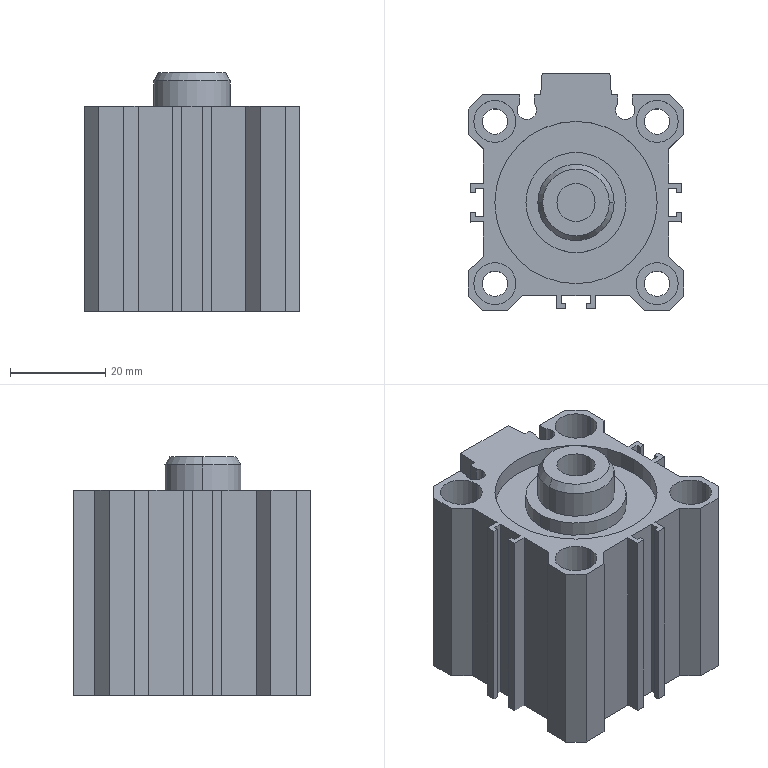Part | STEP file | Air Cylinder CQ2B32-30D | 1 solid | 145 faces | box 45.2 x 49.7 x 50 mm | volume 69030 mm3 | plane 95 | cylinder 44 | cone 6 | commonest cylinder face diameters 8.8 x16 5.3 x8 4 x6 8.5 x4 8 x2 16 x2